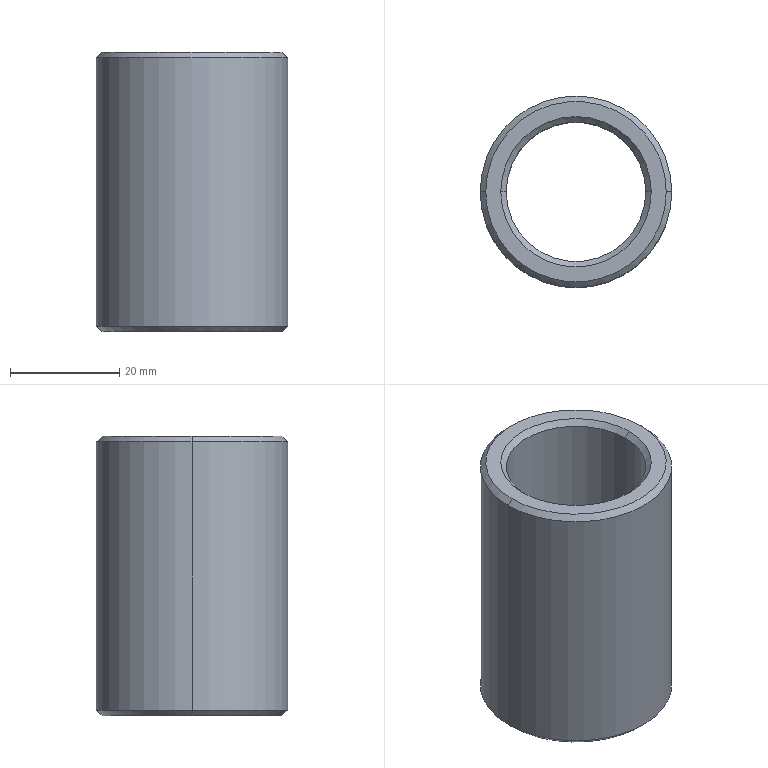Part | SolidWorks | features Chamfer 1, Extrusion 1 | 1 solid | 14 faces | box 35 x 35 x 51 mm | volume 22832 mm3 | cone 8 | cylinder 4 | plane 2 | commonest cylinder face diameters 25.5 x2 35 x2
STEP:
#1=CARTESIAN_POINT('',(16.5,0.,25.5));
#2=VERTEX_POINT('',#1);
#3=CARTESIAN_POINT('',(-16.5,0.,25.5));
#4=VERTEX_POINT('',#3);
#5=CARTESIAN_POINT('',(0.,0.,25.5));
#6=DIRECTION('',(0.,0.,1.));
#7=DIRECTION('',(1.,0.,0.));
#8=AXIS2_PLACEMENT_3D('',#5,#6,#7);
#9=CIRCLE('',#8,16.5);
#10=EDGE_CURVE('',#2,#4,#9,.T.);
#11=ORIENTED_EDGE('',*,*,#10,.F.);
#12=CARTESIAN_POINT('',(17.5,0.,24.5));
#13=VERTEX_POINT('',#12);
#14=CARTESIAN_POINT('',(16.5,0.,25.5));
#15=DIRECTION('',(0.7071,0.,-0.7071));
#16=VECTOR('',#15,1000.);
#17=LINE('',#14,#16);
#18=EDGE_CURVE('',#2,#13,#17,.T.);
#19=ORIENTED_EDGE('',*,*,#18,.T.);
#20=CARTESIAN_POINT('',(-17.5,0.,24.5));
#21=VERTEX_POINT('',#20);
#22=CARTESIAN_POINT('',(0.,0.,24.5));
#23=DIRECTION('',(0.,0.,-1.));
#24=DIRECTION('',(1.,0.,0.));
#25=AXIS2_PLACEMENT_3D('',#22,#23,#24);
#26=CIRCLE('',#25,17.5);
#27=EDGE_CURVE('',#21,#13,#26,.T.);
#28=ORIENTED_EDGE('',*,*,#27,.F.);
#29=CARTESIAN_POINT('',(-16.5,0.,25.5));
#30=DIRECTION('',(-0.7071,0.,-0.7071));
#31=VECTOR('',#30,1000.);
#32=LINE('',#29,#31);
#33=EDGE_CURVE('',#4,#21,#32,.T.);
#34=ORIENTED_EDGE('',*,*,#33,.F.);
#35=EDGE_LOOP('',(#11,#19,#28,#34));
#36=FACE_OUTER_BOUND('',#35,.T.);
#37=CARTESIAN_POINT('',(0.,0.,25.5));
#38=DIRECTION('',(0.,0.,-1.));
#39=DIRECTION('',(-1.,0.,0.));
#40=AXIS2_PLACEMENT_3D('',#37,#38,#39);
#41=CONICAL_SURFACE('',#40,16.5,0.7854);
#42=ADVANCED_FACE('',(#36),#41,.T.);
#43=CARTESIAN_POINT('',(-12.75,0.,24.5));
#44=VERTEX_POINT('',#43);
#45=CARTESIAN_POINT('',(12.75,0.,24.5));
#46=VERTEX_POINT('',#45);
#47=CARTESIAN_POINT('',(0.,0.,24.5));
#48=DIRECTION('',(0.,0.,1.));
#49=DIRECTION('',(1.,0.,0.));
#50=AXIS2_PLACEMENT_3D('',#47,#48,#49);
#51=CIRCLE('',#50,12.75);
#52=EDGE_CURVE('',#44,#46,#51,.T.);
#53=ORIENTED_EDGE('',*,*,#52,.F.);
#54=CARTESIAN_POINT('',(-13.75,0.,25.5));
#55=VERTEX_POINT('',#54);
#56=CARTESIAN_POINT('',(-12.75,0.,24.5));
#57=DIRECTION('',(-0.7071,0.,0.7071));
#58=VECTOR('',#57,1000.);
#59=LINE('',#56,#58);
#60=EDGE_CURVE('',#44,#55,#59,.T.);
#61=ORIENTED_EDGE('',*,*,#60,.T.);
#62=CARTESIAN_POINT('',(13.75,0.,25.5));
#63=VERTEX_POINT('',#62);
#64=CARTESIAN_POINT('',(0.,0.,25.5));
#65=DIRECTION('',(0.,0.,-1.));
#66=DIRECTION('',(1.,0.,0.));
#67=AXIS2_PLACEMENT_3D('',#64,#65,#66);
#68=CIRCLE('',#67,13.75);
#69=EDGE_CURVE('',#63,#55,#68,.T.);
#70=ORIENTED_EDGE('',*,*,#69,.F.);
#71=CARTESIAN_POINT('',(12.75,0.,24.5));
#72=DIRECTION('',(0.7071,0.,0.7071));
#73=VECTOR('',#72,1000.);
#74=LINE('',#71,#73);
#75=EDGE_CURVE('',#46,#63,#74,.T.);
#76=ORIENTED_EDGE('',*,*,#75,.F.);
#77=EDGE_LOOP('',(#53,#61,#70,#76));
#78=FACE_OUTER_BOUND('',#77,.T.);
#79=CARTESIAN_POINT('',(0.,0.,24.5));
#80=DIRECTION('',(0.,0.,1.));
#81=DIRECTION('',(1.,0.,0.));
#82=AXIS2_PLACEMENT_3D('',#79,#80,#81);
#83=CONICAL_SURFACE('',#82,12.75,0.7854);
#84=ADVANCED_FACE('',(#78),#83,.F.);
#85=CARTESIAN_POINT('',(12.75,0.,-24.5));
#86=VERTEX_POINT('',#85);
#87=CARTESIAN_POINT('',(-12.75,0.,-24.5));
#88=VERTEX_POINT('',#87);
#89=CARTESIAN_POINT('',(0.,0.,-24.5));
#90=DIRECTION('',(0.,0.,-1.));
#91=DIRECTION('',(1.,0.,0.));
#92=AXIS2_PLACEMENT_3D('',#89,#90,#91);
#93=CIRCLE('',#92,12.75);
#94=EDGE_CURVE('',#86,#88,#93,.T.);
#95=ORIENTED_EDGE('',*,*,#94,.F.);
#96=CARTESIAN_POINT('',(13.75,0.,-25.5));
#97=VERTEX_POINT('',#96);
#98=CARTESIAN_POINT('',(13.75,0.,-25.5));
#99=DIRECTION('',(0.7071,0.,-0.7071));
#100=VECTOR('',#99,1000.);
#101=LINE('',#98,#100);
#102=EDGE_CURVE('',#86,#97,#101,.T.);
#103=ORIENTED_EDGE('',*,*,#102,.T.);
#104=CARTESIAN_POINT('',(-13.75,0.,-25.5));
#105=VERTEX_POINT('',#104);
#106=CARTESIAN_POINT('',(0.,0.,-25.5));
#107=DIRECTION('',(0.,0.,1.));
#108=DIRECTION('',(1.,0.,0.));
#109=AXIS2_PLACEMENT_3D('',#106,#107,#108);
#110=CIRCLE('',#109,13.75);
#111=EDGE_CURVE('',#105,#97,#110,.T.);
#112=ORIENTED_EDGE('',*,*,#111,.F.);
#113=CARTESIAN_POINT('',(-13.75,0.,-25.5));
#114=DIRECTION('',(-0.7071,0.,-0.7071));
#115=VECTOR('',#114,1000.);
#116=LINE('',#113,#115);
#117=EDGE_CURVE('',#88,#105,#116,.T.);
#118=ORIENTED_EDGE('',*,*,#117,.F.);
#119=EDGE_LOOP('',(#95,#103,#112,#118));
#120=FACE_OUTER_BOUND('',#119,.T.);
#121=CARTESIAN_POINT('',(0.,0.,-25.5));
#122=DIRECTION('',(0.,0.,-1.));
#123=DIRECTION('',(-1.,0.,0.));
#124=AXIS2_PLACEMENT_3D('',#121,#122,#123);
#125=CONICAL_SURFACE('',#124,13.75,0.7854);
#126=ADVANCED_FACE('',(#120),#125,.F.);
#127=CARTESIAN_POINT('',(-16.5,0.,-25.5));
#128=VERTEX_POINT('',#127);
#129=CARTESIAN_POINT('',(16.5,0.,-25.5));
#130=VERTEX_POINT('',#129);
#131=CARTESIAN_POINT('',(0.,0.,-25.5));
#132=DIRECTION('',(0.,0.,-1.));
#133=DIRECTION('',(1.,0.,0.));
#134=AXIS2_PLACEMENT_3D('',#131,#132,#133);
#135=CIRCLE('',#134,16.5);
#136=EDGE_CURVE('',#128,#130,#135,.T.);
#137=ORIENTED_EDGE('',*,*,#136,.F.);
#138=CARTESIAN_POINT('',(-17.5,0.,-24.5));
#139=VERTEX_POINT('',#138);
#140=CARTESIAN_POINT('',(-17.5,0.,-24.5));
#141=DIRECTION('',(-0.7071,0.,0.7071));
#142=VECTOR('',#141,1000.);
#143=LINE('',#140,#142);
#144=EDGE_CURVE('',#128,#139,#143,.T.);
#145=ORIENTED_EDGE('',*,*,#144,.T.);
#146=CARTESIAN_POINT('',(17.5,0.,-24.5));
#147=VERTEX_POINT('',#146);
#148=CARTESIAN_POINT('',(0.,0.,-24.5));
#149=DIRECTION('',(0.,0.,1.));
#150=DIRECTION('',(1.,0.,0.));
#151=AXIS2_PLACEMENT_3D('',#148,#149,#150);
#152=CIRCLE('',#151,17.5);
#153=EDGE_CURVE('',#147,#139,#152,.T.);
#154=ORIENTED_EDGE('',*,*,#153,.F.);
#155=CARTESIAN_POINT('',(17.5,0.,-24.5));
#156=DIRECTION('',(0.7071,0.,0.7071));
#157=VECTOR('',#156,1000.);
#158=LINE('',#155,#157);
#159=EDGE_CURVE('',#130,#147,#158,.T.);
#160=ORIENTED_EDGE('',*,*,#159,.F.);
#161=EDGE_LOOP('',(#137,#145,#154,#160));
#162=FACE_OUTER_BOUND('',#161,.T.);
#163=CARTESIAN_POINT('',(0.,0.,-24.5));
#164=DIRECTION('',(0.,0.,1.));
#165=DIRECTION('',(1.,0.,0.));
#166=AXIS2_PLACEMENT_3D('',#163,#164,#165);
#167=CONICAL_SURFACE('',#166,17.5,0.7854);
#168=ADVANCED_FACE('',(#162),#167,.T.);
#169=ORIENTED_EDGE('',*,*,#52,.T.);
#170=CARTESIAN_POINT('',(12.75,0.,25.5));
#171=DIRECTION('',(0.,0.,-1.));
#172=VECTOR('',#171,1000.);
#173=LINE('',#170,#172);
#174=EDGE_CURVE('',#46,#86,#173,.T.);
#175=ORIENTED_EDGE('',*,*,#174,.T.);
#176=ORIENTED_EDGE('',*,*,#94,.T.);
#177=CARTESIAN_POINT('',(-12.75,0.,25.5));
#178=DIRECTION('',(0.,0.,-1.));
#179=VECTOR('',#178,1000.);
#180=LINE('',#177,#179);
#181=EDGE_CURVE('',#44,#88,#180,.T.);
#182=ORIENTED_EDGE('',*,*,#181,.F.);
#183=EDGE_LOOP('',(#169,#175,#176,#182));
#184=FACE_OUTER_BOUND('',#183,.T.);
#185=CARTESIAN_POINT('',(0.,0.,25.5));
#186=DIRECTION('',(0.,0.,-1.));
#187=DIRECTION('',(-1.,0.,0.));
#188=AXIS2_PLACEMENT_3D('',#185,#186,#187);
#189=CYLINDRICAL_SURFACE('',#188,12.75);
#190=ADVANCED_FACE('',(#184),#189,.F.);
#191=ORIENTED_EDGE('',*,*,#27,.T.);
#192=CARTESIAN_POINT('',(17.5,0.,25.5));
#193=DIRECTION('',(0.,0.,-1.));
#194=VECTOR('',#193,1000.);
#195=LINE('',#192,#194);
#196=EDGE_CURVE('',#13,#147,#195,.T.);
#197=ORIENTED_EDGE('',*,*,#196,.T.);
#198=ORIENTED_EDGE('',*,*,#153,.T.);
#199=CARTESIAN_POINT('',(-17.5,0.,25.5));
#200=DIRECTION('',(0.,0.,-1.));
#201=VECTOR('',#200,1000.);
#202=LINE('',#199,#201);
#203=EDGE_CURVE('',#21,#139,#202,.T.);
#204=ORIENTED_EDGE('',*,*,#203,.F.);
#205=EDGE_LOOP('',(#191,#197,#198,#204));
#206=FACE_OUTER_BOUND('',#205,.T.);
#207=CARTESIAN_POINT('',(0.,0.,25.5));
#208=DIRECTION('',(0.,0.,-1.));
#209=DIRECTION('',(-1.,0.,0.));
#210=AXIS2_PLACEMENT_3D('',#207,#208,#209);
#211=CYLINDRICAL_SURFACE('',#210,17.5);
#212=ADVANCED_FACE('',(#206),#211,.T.);
#213=ORIENTED_EDGE('',*,*,#69,.T.);
#214=CARTESIAN_POINT('',(0.,0.,25.5));
#215=DIRECTION('',(0.,0.,-1.));
#216=DIRECTION('',(1.,0.,0.));
#217=AXIS2_PLACEMENT_3D('',#214,#215,#216);
#218=CIRCLE('',#217,13.75);
#219=EDGE_CURVE('',#55,#63,#218,.T.);
#220=ORIENTED_EDGE('',*,*,#219,.T.);
#221=EDGE_LOOP('',(#213,#220));
#222=FACE_BOUND('',#221,.T.);
#223=CARTESIAN_POINT('',(0.,0.,25.5));
#224=DIRECTION('',(0.,0.,1.));
#225=DIRECTION('',(1.,0.,0.));
#226=AXIS2_PLACEMENT_3D('',#223,#224,#225);
#227=CIRCLE('',#226,16.5);
#228=EDGE_CURVE('',#4,#2,#227,.T.);
#229=ORIENTED_EDGE('',*,*,#228,.T.);
#230=ORIENTED_EDGE('',*,*,#10,.T.);
#231=EDGE_LOOP('',(#229,#230));
#232=FACE_OUTER_BOUND('',#231,.T.);
#233=CARTESIAN_POINT('',(0.,0.,25.5));
#234=DIRECTION('',(0.,0.,1.));
#235=DIRECTION('',(1.,0.,0.));
#236=AXIS2_PLACEMENT_3D('',#233,#234,#235);
#237=PLANE('',#236);
#238=ADVANCED_FACE('',(#222,#232),#237,.T.);
#239=CARTESIAN_POINT('',(0.,0.,-25.5));
#240=DIRECTION('',(0.,0.,-1.));
#241=DIRECTION('',(1.,0.,0.));
#242=AXIS2_PLACEMENT_3D('',#239,#240,#241);
#243=CIRCLE('',#242,16.5);
#244=EDGE_CURVE('',#130,#128,#243,.T.);
#245=ORIENTED_EDGE('',*,*,#244,.T.);
#246=ORIENTED_EDGE('',*,*,#136,.T.);
#247=EDGE_LOOP('',(#245,#246));
#248=FACE_OUTER_BOUND('',#247,.T.);
#249=ORIENTED_EDGE('',*,*,#111,.T.);
#250=CARTESIAN_POINT('',(0.,0.,-25.5));
#251=DIRECTION('',(0.,0.,1.));
#252=DIRECTION('',(1.,0.,0.));
#253=AXIS2_PLACEMENT_3D('',#250,#251,#252);
#254=CIRCLE('',#253,13.75);
#255=EDGE_CURVE('',#97,#105,#254,.T.);
#256=ORIENTED_EDGE('',*,*,#255,.T.);
#257=EDGE_LOOP('',(#249,#256));
#258=FACE_BOUND('',#257,.T.);
#259=CARTESIAN_POINT('',(0.,0.,-25.5));
#260=DIRECTION('',(0.,0.,1.));
#261=DIRECTION('',(1.,0.,0.));
#262=AXIS2_PLACEMENT_3D('',#259,#260,#261);
#263=PLANE('',#262);
#264=ADVANCED_FACE('',(#248,#258),#263,.F.);
#265=ORIENTED_EDGE('',*,*,#196,.F.);
#266=CARTESIAN_POINT('',(0.,0.,24.5));
#267=DIRECTION('',(0.,0.,-1.));
#268=DIRECTION('',(1.,0.,0.));
#269=AXIS2_PLACEMENT_3D('',#266,#267,#268);
#270=CIRCLE('',#269,17.5);
#271=EDGE_CURVE('',#13,#21,#270,.T.);
#272=ORIENTED_EDGE('',*,*,#271,.T.);
#273=ORIENTED_EDGE('',*,*,#203,.T.);
#274=CARTESIAN_POINT('',(0.,0.,-24.5));
#275=DIRECTION('',(0.,0.,1.));
#276=DIRECTION('',(1.,0.,0.));
#277=AXIS2_PLACEMENT_3D('',#274,#275,#276);
#278=CIRCLE('',#277,17.5);
#279=EDGE_CURVE('',#139,#147,#278,.T.);
#280=ORIENTED_EDGE('',*,*,#279,.T.);
#281=EDGE_LOOP('',(#265,#272,#273,#280));
#282=FACE_OUTER_BOUND('',#281,.T.);
#283=CARTESIAN_POINT('',(0.,0.,25.5));
#284=DIRECTION('',(0.,0.,-1.));
#285=DIRECTION('',(-1.,0.,0.));
#286=AXIS2_PLACEMENT_3D('',#283,#284,#285);
#287=CYLINDRICAL_SURFACE('',#286,17.5);
#288=ADVANCED_FACE('',(#282),#287,.T.);
#289=ORIENTED_EDGE('',*,*,#174,.F.);
#290=CARTESIAN_POINT('',(0.,0.,24.5));
#291=DIRECTION('',(0.,0.,1.));
#292=DIRECTION('',(1.,0.,0.));
#293=AXIS2_PLACEMENT_3D('',#290,#291,#292);
#294=CIRCLE('',#293,12.75);
#295=EDGE_CURVE('',#46,#44,#294,.T.);
#296=ORIENTED_EDGE('',*,*,#295,.T.);
#297=ORIENTED_EDGE('',*,*,#181,.T.);
#298=CARTESIAN_POINT('',(0.,0.,-24.5));
#299=DIRECTION('',(0.,0.,-1.));
#300=DIRECTION('',(1.,0.,0.));
#301=AXIS2_PLACEMENT_3D('',#298,#299,#300);
#302=CIRCLE('',#301,12.75);
#303=EDGE_CURVE('',#88,#86,#302,.T.);
#304=ORIENTED_EDGE('',*,*,#303,.T.);
#305=EDGE_LOOP('',(#289,#296,#297,#304));
#306=FACE_OUTER_BOUND('',#305,.T.);
#307=CARTESIAN_POINT('',(0.,0.,25.5));
#308=DIRECTION('',(0.,0.,-1.));
#309=DIRECTION('',(-1.,0.,0.));
#310=AXIS2_PLACEMENT_3D('',#307,#308,#309);
#311=CYLINDRICAL_SURFACE('',#310,12.75);
#312=ADVANCED_FACE('',(#306),#311,.F.);
#313=ORIENTED_EDGE('',*,*,#144,.F.);
#314=ORIENTED_EDGE('',*,*,#244,.F.);
#315=ORIENTED_EDGE('',*,*,#159,.T.);
#316=ORIENTED_EDGE('',*,*,#279,.F.);
#317=EDGE_LOOP('',(#313,#314,#315,#316));
#318=FACE_OUTER_BOUND('',#317,.T.);
#319=CARTESIAN_POINT('',(0.,0.,-24.5));
#320=DIRECTION('',(0.,0.,1.));
#321=DIRECTION('',(1.,0.,0.));
#322=AXIS2_PLACEMENT_3D('',#319,#320,#321);
#323=CONICAL_SURFACE('',#322,17.5,0.7854);
#324=ADVANCED_FACE('',(#318),#323,.T.);
#325=ORIENTED_EDGE('',*,*,#102,.F.);
#326=ORIENTED_EDGE('',*,*,#303,.F.);
#327=ORIENTED_EDGE('',*,*,#117,.T.);
#328=ORIENTED_EDGE('',*,*,#255,.F.);
#329=EDGE_LOOP('',(#325,#326,#327,#328));
#330=FACE_OUTER_BOUND('',#329,.T.);
#331=CARTESIAN_POINT('',(0.,0.,-25.5));
#332=DIRECTION('',(0.,0.,-1.));
#333=DIRECTION('',(-1.,0.,0.));
#334=AXIS2_PLACEMENT_3D('',#331,#332,#333);
#335=CONICAL_SURFACE('',#334,13.75,0.7854);
#336=ADVANCED_FACE('',(#330),#335,.F.);
#337=ORIENTED_EDGE('',*,*,#60,.F.);
#338=ORIENTED_EDGE('',*,*,#295,.F.);
#339=ORIENTED_EDGE('',*,*,#75,.T.);
#340=ORIENTED_EDGE('',*,*,#219,.F.);
#341=EDGE_LOOP('',(#337,#338,#339,#340));
#342=FACE_OUTER_BOUND('',#341,.T.);
#343=CARTESIAN_POINT('',(0.,0.,24.5));
#344=DIRECTION('',(0.,0.,1.));
#345=DIRECTION('',(1.,0.,0.));
#346=AXIS2_PLACEMENT_3D('',#343,#344,#345);
#347=CONICAL_SURFACE('',#346,12.75,0.7854);
#348=ADVANCED_FACE('',(#342),#347,.F.);
#349=ORIENTED_EDGE('',*,*,#18,.F.);
#350=ORIENTED_EDGE('',*,*,#228,.F.);
#351=ORIENTED_EDGE('',*,*,#33,.T.);
#352=ORIENTED_EDGE('',*,*,#271,.F.);
#353=EDGE_LOOP('',(#349,#350,#351,#352));
#354=FACE_OUTER_BOUND('',#353,.T.);
#355=CARTESIAN_POINT('',(0.,0.,25.5));
#356=DIRECTION('',(0.,0.,-1.));
#357=DIRECTION('',(-1.,0.,0.));
#358=AXIS2_PLACEMENT_3D('',#355,#356,#357);
#359=CONICAL_SURFACE('',#358,16.5,0.7854);
#360=ADVANCED_FACE('',(#354),#359,.T.);
#361=CLOSED_SHELL('',(#42,#84,#126,#168,#190,#212,#238,#264,#288,#312,#324,#336,#348,#360));
#362=MANIFOLD_SOLID_BREP('',#361);
#363=CARTESIAN_POINT('',(0.,0.,0.));
#364=DIRECTION('',(0.,0.,1.));
#365=DIRECTION('',(1.,0.,0.));
#366=AXIS2_PLACEMENT_3D('',#363,#364,#365);
#367=(LENGTH_UNIT()NAMED_UNIT(*)SI_UNIT(.MILLI.,.METRE.));
#368=UNCERTAINTY_MEASURE_WITH_UNIT(LENGTH_MEASURE(0.00001),#367,'','');
#369=(NAMED_UNIT(*)PLANE_ANGLE_UNIT()SI_UNIT($,.RADIAN.));
#370=(NAMED_UNIT(*)SI_UNIT($,.STERADIAN.)SOLID_ANGLE_UNIT());
#371=(GEOMETRIC_REPRESENTATION_CONTEXT(3)GLOBAL_UNCERTAINTY_ASSIGNED_CONTEXT((#368))GLOBAL_UNIT_ASSIGNED_CONTEXT((#367,#369,#370))REPRESENTATION_CONTEXT('',''));
#372=ADVANCED_BREP_SHAPE_REPRESENTATION('',(#362,#366),#371);